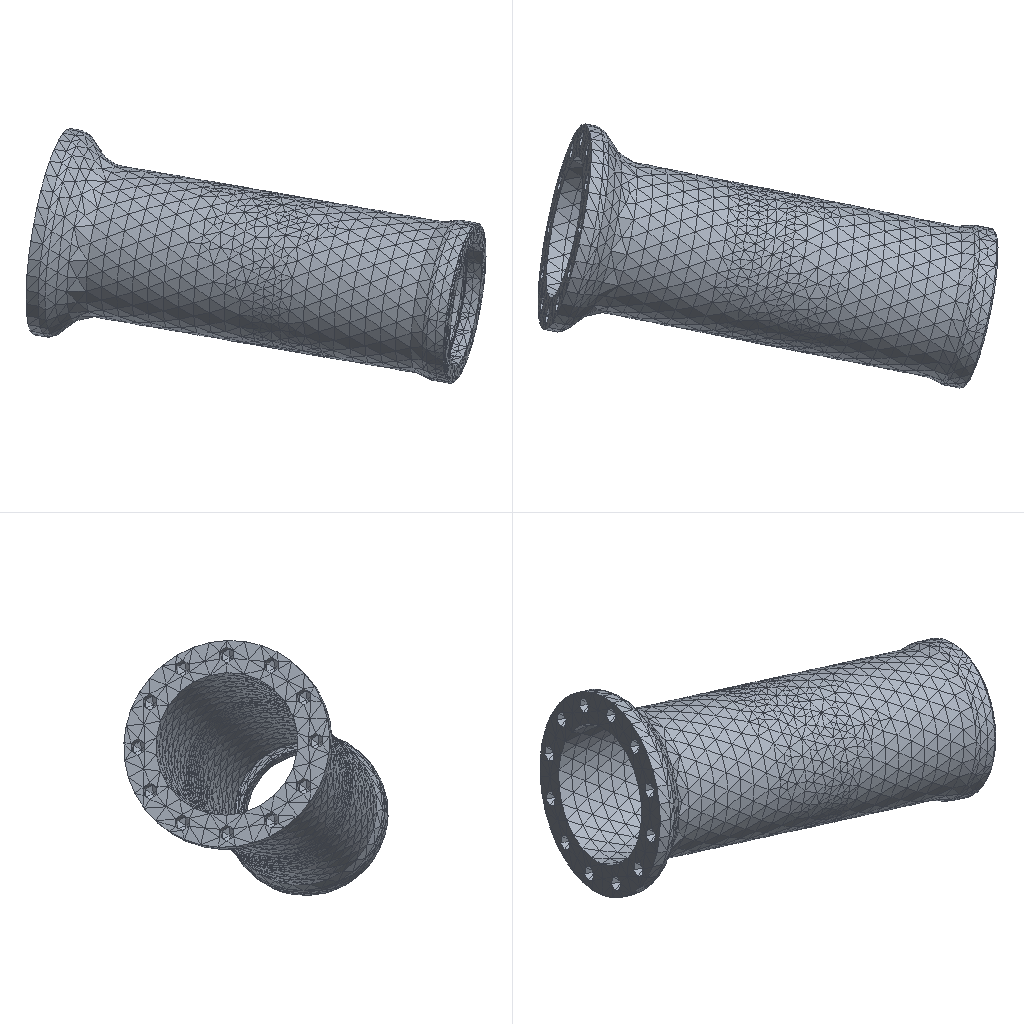Simulation study | ansys workbench
Set-up summary:
category,name,step,type,value,unit,region
solver,ansys_workbench
units,mm-N-s-tonne (MPa),,stated,"/units,MPA"
analysis,LS1,,transient
load_step,LS1,LS1,transient,time=0.171
mesh,nodes,,,3014
mesh,elements,,,9796
element_type,SOLID185,,,9455
element_type,CONTA174,,,341
material,moduan,,E,210000,tonne s^-2 mm^-1
material,moduan,,nu,0.3
material,moduan,,density,7.85e-09,tonne mm^-3
material,joint_1,,E,210000,tonne s^-2 mm^-1
material,joint_1,,nu,0.3
material,joint_1,,density,9.34279e-10,tonne mm^-3
material,link,,E,69000,tonne s^-2 mm^-1
material,link,,nu,0.3
material,link,,density,2.7e-09,tonne mm^-3
material,joint_4,,E,210000,tonne s^-2 mm^-1
material,joint_4,,nu,0.3
material,joint_4,,density,2.47283e-09,tonne mm^-3
material,joint_5,,E,210000,tonne s^-2 mm^-1
material,joint_5,,nu,0.3
material,joint_5,,density,1.91585e-09,tonne mm^-3
material,joint_6,,E,210000,tonne s^-2 mm^-1
material,joint_6,,nu,0.3
material,joint_6,,density,2.14316e-09,tonne mm^-3
material,joint_3,,E,210000,tonne s^-2 mm^-1
material,joint_3,,nu,0.3
material,joint_3,,density,1.46252e-09,tonne mm^-3
material,jpint_2,,E,210000,tonne s^-2 mm^-1
material,jpint_2,,nu,0.3
material,jpint_2,,density,1.01587e-08,tonne mm^-3
load,ACEL,LS1,gravity (ACEL; gravity acts opposite),"9806.65 [dir=(0, -1, 0)]",,all
bc,,LS1,fixed,"[dofs=ROTX,ROTY,ROTZ,UX,UY,UZ n=6]",,node list
contact,contact 1,,bonded (always),element=CONTA174
contact,contact 2,,bonded (always),element=CONTA174
named_set,REMOTEDISPALL,,node,1
Ansys APDL input file, long lists of numbers shortened:
/batch
/config,noeldb,1     ! force off writing results to database
*get,_wallstrt,active,,time,wall
! ANSYS input file written by Workbench version 2020 R2
! File used for geometry attach:
/title,UR16e--Transient (A5)
*DIM,_wb_ProjectScratch_dir,string,248
_wb_ProjectScratch_dir(1) = ''
*DIM,_wb_SolverFiles_dir,string,248
_wb_SolverFiles_dir(1) = ''
*DIM,_wb_userfiles_dir,string,248
_wb_userfiles_dir(1) = ''
/com,--- Data in consistent NMM units. See Solving Units in the help system for more information.
/units,MPA
/nopr
/wb,file,start              !  signify a WB generated input file
/prep7
! Turn off shape checking because checks already performed inside WB mesher.
! See help system for more information.
SHPP,OFF,,NOWARN
/nolist
etcon,set             ! allow ANSYS to choose best KEYOP's for 180x elements
/com,*********** Nodes for the whole assembly ***********
nblock,3,,3291
(1i9,3e20.9e3)
     2990    -2.619038221E+02     6.000698852E+02    -1.306205958E+02
! (2991 more lines like these left out)
-1
/com,*********** Nodes for all Remote Points ***********
nblock,3
(1i9,3e20.9e3)
   114271     1.429985942E-14     1.067999974E+02     1.194186063E-13
! (21 more lines like these left out)
-1
/wb,elem,start            !  set before creation of elements
/com,*********** Elements for Body 1 "base" ***********
/com,*********** Send Body as a Rigid Body ***********
et,1,21
keyo,1,2,1             ! Moments of inertia in nodal coordinates
keyo,1,3,0         ! 3D Mass With Rotary Intertia
r,1,1.02367975074938e-002,1.02367975074938e-002,1.02367975074938e-002,26.633,39.557,29.838
local,11,0,7.8090358886332e-002,63.831,-1.168,-0.1084,-3.09,0.1323
nrot,1
csys,0
mat,1
real,1
type,1
en,15078,1
/com,*********** Elements for Body 2 "joint_1" ***********
/com,*********** Send Body as a Rigid Body ***********
et,2,21
keyo,2,2,1             ! Moments of inertia in nodal coordinates
keyo,2,3,0         ! 3D Mass With Rotary Intertia
r,2,3.19999436398941e-003,3.19999436398941e-003,3.19999436398941e-003,13.065,11.645,10.957
local,11,0,-2.749,184.232,-15.857,-0.9454,5.268,9.901
nrot,2
csys,0
mat,2
real,2
type,2
en,15079,2
/com,*********** Elements for Body 3 "link_3" ***********
et,3,185
eblock,19,solid,,9455
(19i9)
        3        3        3        3        0        0        0        0        8        0        1      629     2969     1014     1014      630      630      630      630
! (9454 more lines like these left out)
-1
/com,*********** Elements for Body 4 "Link_2" ***********
/com,*********** Send Body as a Rigid Body ***********
et,4,21
keyo,4,2,1             ! Moments of inertia in nodal coordinates
keyo,4,3,0         ! 3D Mass With Rotary Intertia
r,4,8.50492430756376e-004,8.50492430756376e-004,8.50492430756376e-004,2.049,2.57,2.908
local,11,0,-233.317,606.482,-20.639,-10.872,-1.872,-37.264
nrot,2985
csys,0
mat,4
real,4
type,4
en,15080,2985
/com,*********** Elements for Body 5 "jpint_4" ***********
/com,*********** Send Body as a Rigid Body ***********
et,5,21
keyo,5,2,1             ! Moments of inertia in nodal coordinates
keyo,5,3,0         ! 3D Mass With Rotary Intertia
r,5,1.79999317481185e-003,1.79999317481185e-003,1.79999317481185e-003,2.575,2.69,2.136
local,11,0,99.549,541.334,-55.788,-10.802,-1.885,3.272
nrot,2986
csys,0
mat,5
real,5
type,5
en,15081,2986
/com,*********** Elements for Body 6 "joint_5" ***********
/com,*********** Send Body as a Rigid Body ***********
et,6,21
keyo,6,2,1             ! Moments of inertia in nodal coordinates
keyo,6,3,0         ! 3D Mass With Rotary Intertia
r,6,1.79999426944407e-003,1.79999426944407e-003,1.79999426944407e-003,3.487,3.061,2.341
local,11,0,83.755,539.911,-172.299,-41.598,-4.879,7.34
nrot,2987
csys,0
mat,6
real,6
type,6
en,15082,2987
/com,*********** Elements for Body 7 "joint_6" ***********
/com,*********** Send Body as a Rigid Body ***********
et,7,21
keyo,7,2,1             ! Moments of inertia in nodal coordinates
keyo,7,3,0         ! 3D Mass With Rotary Intertia
r,7,1.799990079675e-003,1.799990079675e-003,1.799990079675e-003,2.398,2.565,3.034
local,11,0,151.28,621.209,-202.996,36.251,5.214,7.789
nrot,2988
csys,0
mat,7
real,7
type,7
en,15083,2988
/com,*********** Elements for Body 8 "moduan" ***********
/com,*********** Send Body as a Rigid Body ***********
et,8,21
keyo,8,2,1             ! Moments of inertia in nodal coordinates
keyo,8,3,0         ! 3D Mass With Rotary Intertia
r,8,2.97368674504464e-003,2.97368674504464e-003,2.97368674504464e-003,2.801,2.33,2.336
local,11,0,220.284,574.903,-213.956,-38.665,-27.596,7.642
nrot,2989
csys,0
mat,8
real,8
type,8
en,15084,2989
/com,*********** Elements for Body 9 "joint_3" ***********
/com,*********** Send Body as a Rigid Body ***********
et,9,21
keyo,9,2,1             ! Moments of inertia in nodal coordinates
keyo,9,3,0         ! 3D Mass With Rotary Intertia
r,9,2.40005206162437e-003,2.40005206162437e-003,2.40005206162437e-003,5.964,5.358,4.799
local,11,0,-261.904,600.07,-130.621,32.525,-18.283,9.006
nrot,2990
csys,0
mat,9
real,9
type,9
en,15085,2990
/com,*********** Elements for Body 10 "joint_2" ***********
/com,*********** Send Body as a Rigid Body ***********
et,10,21
keyo,10,2,1             ! Moments of inertia in nodal coordinates
keyo,10,3,0         ! 3D Mass With Rotary Intertia
r,10,3.06619312289427e-002,3.06619312289427e-002,3.06619312289427e-002,112.393,110.597,96.78
local,11,0,-33.808,186.218,-176.77,27.519,12.66,8.86
nrot,2991
csys,0
mat,10
real,10
type,10
en,15086,2991
/com,*********** Elements for Body 11 "Link_1" ***********
/com,*********** Send Body as a Rigid Body ***********
et,11,21
keyo,11,2,1             ! Moments of inertia in nodal coordinates
keyo,11,3,0         ! 3D Mass With Rotary Intertia
r,11,2.24521379583667e-003,2.24521379583667e-003,2.24521379583667e-003,34.363,6.799,34.363
local,11,0,-138.935,377.254,-154.531,28.98,4.803,0.4433
nrot,2992
csys,0
mat,11
real,11
type,11
en,15087,2992
/wb,elem,end               !  done creating elements
/com,*********** Send User Defined Coordinate System(s) ***********
local,12,0,1.42998594161399e-014,106.8,1.19418606342056e-013,5.518,-90.,5.518
local,13,0,-17.447,180.7,-100.598,-1.26833640216353e-014,9.7869357942221e-014,9.839
local,14,0,-255.778,609.325,-64.845,-1.19904740548723e-015,4.20102064352059e-013,9.839
local,15,0,95.681,540.401,-106.111,-7.6091083357917e-015,1.34257806861156e-013,9.839
local,16,0,113.452,577.213,-196.426,180.,-81.305,-138.924
local,17,0,196.105,596.769,-210.196,-180.,80.114,-132.6
local,18,0,-68.796,250.612,-166.696,99.269,-76.01,69.735
local,19,0,-231.933,545.166,-138.402,-1.12265577235347e-013,-84.513,-28.868
local,20,0,-175.359,595.732,-8.966,173.246,24.487,-100.62
local,21,0,52.965,550.529,-48.565,-180.,48.78,-104.746
local,22,0,240.749,556.326,-217.244,-87.35,80.633,135.561
csys,0
toffst,273.15,  ! Temperature offset from absolute zero
/com,*********** Set Reference Temperature ***********
tref,22.
/wb,mat,start              !  starting to send materials
/com,*********** Send Materials ***********
MP,DENS,1,7.85e-09,	! tonne mm^-3
MP,EX,1,210000,	! tonne s^-2 mm^-1
MP,NUXY,1,0.3,
MP,DENS,2,9.34279e-10,	! tonne mm^-3
! (29 more lines like these left out)
/wb,mat,end                !  done sending materials
!************************* Model Summary ********************
!base,	moduan,	matid,	1
!joint_1,	joint_1,	matid,	2
!link_3,	link,	matid,	3
!Link_2,	link,	matid,	4
!jpint_4,	joint_4,	matid,	5
!joint_5,	joint_5,	matid,	6
!joint_6,	joint_6,	matid,	7
!moduan,	moduan,	matid,	8
!joint_3,	joint_3,	matid,	9
!joint_2,	jpint_2,	matid,	10
!Link_1,	link,	matid,	11
!************************* End Model Summary ********************
! get the diagonal of the bounding box. Needed later for other things
*get,_xmin,node,,mnloc,x
*get,_ymin,node,,mnloc,y
*get,_zmin,node,,mnloc,z
*get,_xmax,node,,mxloc,x
*get,_ymax,node,,mxloc,y
*get,_zmax,node,,mxloc,z
_ASMDIAG=(_xmax-_xmin)*(_xmax-_xmin)+(_ymax-_ymin)*(_ymax-_ymin)+(_zmax-_zmin)*(_zmax-_zmin)
_ASMDIAG=SQRT(_ASMDIAG)
/wb,contact,start          !  starting to send contact
/wb,contact,end            !  done creating contacts
/golist
/wb,load,start             !  starting to send loads
/com,*********** Create Remote Point "Internal Remote Point" ***********
! -------- Remote Point Used by "Revolute - base To joint_1" --------
! ********* Create Contact to Connect To Rigid Body Mass Node ***********
*set,tid,12
*set,cid,12
et,tid,170
keyo,tid,2,1           ! Set MPC target element and not fix pilot
keyo,tid,4,0           ! Create CE's for all DOFs
type,tid
mat ,cid
real,cid
tshape,pilo
en,613392,1
tshape
! ********* End of Create Contact to Connect To Rigid Body Mass Node ***********
*set,_npilot,114271
_npilot109=_npilot
mat,12
real,12
type,12
en,613393,1,114271
csys,12
nrot,114271
csys,0
/com,*********** Create Remote Point "Internal Remote Point 2" ***********
! -------- Remote Point Used by "Revolute - base To joint_1" --------
! ********* Create Contact to Connect To Rigid Body Mass Node ***********
*set,tid,13
*set,cid,13
et,tid,170
keyo,tid,2,1           ! Set MPC target element and not fix pilot
keyo,tid,4,0           ! Create CE's for all DOFs
type,tid
mat ,cid
real,cid
tshape,pilo
en,613394,2
tshape
! ********* End of Create Contact to Connect To Rigid Body Mass Node ***********
*set,_npilot,114272
_npilot110=_npilot
mat,13
real,13
type,13
en,613395,2,114272
csys,12
nrot,114272
csys,0
/com,*********** Create Remote Point "Internal Remote Point 3" ***********
! -------- Remote Point Used by "Revolute - joint_1 To joint_2" --------
*set,_npilot,114273
_npilot113=_npilot
mat,13
real,13
type,13
en,613396,2,114273
csys,13
nrot,114273
csys,0
/com,*********** Create Remote Point "Internal Remote Point 4" ***********
! -------- Remote Point Used by "Revolute - joint_1 To joint_2" --------
! ********* Create Contact to Connect To Rigid Body Mass Node ***********
*set,tid,14
*set,cid,14
et,tid,170
keyo,tid,2,1           ! Set MPC target element and not fix pilot
keyo,tid,4,0           ! Create CE's for all DOFs
type,tid
mat ,cid
real,cid
tshape,pilo
en,613397,2991
tshape
! ********* End of Create Contact to Connect To Rigid Body Mass Node ***********
*set,_npilot,114274
_npilot114=_npilot
mat,14
real,14
type,14
en,613398,2991,114274
csys,13
nrot,114274
csys,0
/com,*********** Create Remote Point "Internal Remote Point 5" ***********
! -------- Remote Point Used by "Revolute - joint_3 To Link_2" --------
! ********* Create Contact to Connect To Rigid Body Mass Node ***********
*set,tid,15
*set,cid,15
et,tid,170
keyo,tid,2,1           ! Set MPC target element and not fix pilot
keyo,tid,4,0           ! Create CE's for all DOFs
type,tid
mat ,cid
real,cid
tshape,pilo
en,613399,2990
tshape
! ********* End of Create Contact to Connect To Rigid Body Mass Node ***********
*set,_npilot,114275
_npilot117=_npilot
mat,15
real,15
type,15
en,613400,2990,114275
csys,14
nrot,114275
csys,0
/com,*********** Create Remote Point "Internal Remote Point 6" ***********
! -------- Remote Point Used by "Revolute - joint_3 To Link_2" --------
! ********* Create Contact to Connect To Rigid Body Mass Node ***********
*set,tid,16
*set,cid,16
et,tid,170
keyo,tid,2,1           ! Set MPC target element and not fix pilot
keyo,tid,4,0           ! Create CE's for all DOFs
type,tid
mat ,cid
real,cid
tshape,pilo
en,613401,2985
tshape
! ********* End of Create Contact to Connect To Rigid Body Mass Node ***********
*set,_npilot,114276
_npilot118=_npilot
mat,16
real,16
type,16
en,613402,2985,114276
csys,14
nrot,114276
csys,0
/com,*********** Create Remote Point "Internal Remote Point 7" ***********
! -------- Remote Point Used by "Revolute - jpint_4 To joint_5" --------
! ********* Create Contact to Connect To Rigid Body Mass Node ***********
*set,tid,17
*set,cid,17
et,tid,170
keyo,tid,2,1           ! Set MPC target element and not fix pilot
keyo,tid,4,0           ! Create CE's for all DOFs
type,tid
mat ,cid
real,cid
tshape,pilo
en,613403,2986
tshape
! ********* End of Create Contact to Connect To Rigid Body Mass Node ***********
*set,_npilot,114277
_npilot121=_npilot
mat,17
real,17
type,17
en,613404,2986,114277
csys,15
nrot,114277
csys,0
/com,*********** Create Remote Point "Internal Remote Point 8" ***********
! -------- Remote Point Used by "Revolute - jpint_4 To joint_5" --------
! ********* Create Contact to Connect To Rigid Body Mass Node ***********
*set,tid,18
*set,cid,18
et,tid,170
keyo,tid,2,1           ! Set MPC target element and not fix pilot
keyo,tid,4,0           ! Create CE's for all DOFs
type,tid
mat ,cid
real,cid
tshape,pilo
en,613405,2987
tshape
! ********* End of Create Contact to Connect To Rigid Body Mass Node ***********
*set,_npilot,114278
_npilot122=_npilot
mat,18
real,18
type,18
en,613406,2987,114278
csys,15
nrot,114278
csys,0
/com,*********** Create Remote Point "Internal Remote Point 9" ***********
! -------- Remote Point Used by "Revolute - joint_5 To joint_6" --------
*set,_npilot,114279
_npilot125=_npilot
mat,18
real,18
type,18
en,613407,2987,114279
csys,16
nrot,114279
csys,0
/com,*********** Create Remote Point "Internal Remote Point 10" ***********
! -------- Remote Point Used by "Revolute - joint_5 To joint_6" --------
! ********* Create Contact to Connect To Rigid Body Mass Node ***********
*set,tid,19
*set,cid,19
et,tid,170
keyo,tid,2,1           ! Set MPC target element and not fix pilot
keyo,tid,4,0           ! Create CE's for all DOFs
type,tid
mat ,cid
real,cid
tshape,pilo
en,613408,2988
tshape
! ********* End of Create Contact to Connect To Rigid Body Mass Node ***********
*set,_npilot,114280
_npilot126=_npilot
mat,19
real,19
type,19
en,613409,2988,114280
csys,16
nrot,114280
csys,0
/com,*********** Create Remote Point "Internal Remote Point 11" ***********
! -------- Remote Point Used by "Revolute - joint_6 To moduan" --------
*set,_npilot,114281
_npilot129=_npilot
mat,19
real,19
type,19
en,613410,2988,114281
csys,17
nrot,114281
csys,0
/com,*********** Create Remote Point "Internal Remote Point 12" ***********
! -------- Remote Point Used by "Revolute - joint_6 To moduan" --------
! ********* Create Contact to Connect To Rigid Body Mass Node ***********
*set,tid,20
*set,cid,20
et,tid,170
keyo,tid,2,1           ! Set MPC target element and not fix pilot
keyo,tid,4,0           ! Create CE's for all DOFs
type,tid
mat ,cid
real,cid
tshape,pilo
en,613411,2989
tshape
! ********* End of Create Contact to Connect To Rigid Body Mass Node ***********
*set,_npilot,114282
_npilot130=_npilot
mat,20
real,20
type,20
en,613412,2989,114282
csys,17
nrot,114282
csys,0
/com,*********** Create Remote Point "Internal Remote Point 13" ***********
! -------- Remote Point Used by "Fixed - joint_2 To Link_1" --------
*set,_npilot,114283
_npilot158=_npilot
mat,14
real,14
type,14
en,613413,2991,114283
csys,18
nrot,114283
csys,0
/com,*********** Create Remote Point "Internal Remote Point 14" ***********
! -------- Remote Point Used by "Fixed - joint_2 To Link_1" --------
! ********* Create Contact to Connect To Rigid Body Mass Node ***********
*set,tid,21
*set,cid,21
et,tid,170
keyo,tid,2,1           ! Set MPC target element and not fix pilot
keyo,tid,4,0           ! Create CE's for all DOFs
type,tid
mat ,cid
real,cid
tshape,pilo
en,613414,2992
tshape
! ********* End of Create Contact to Connect To Rigid Body Mass Node ***********
*set,_npilot,114284
_npilot159=_npilot
mat,21
real,21
type,21
en,613415,2992,114284
csys,18
nrot,114284
csys,0
/com,*********** Create Remote Point "Internal Remote Point 15" ***********
! -------- Remote Point Used by "Fixed - Link_1 To joint_3" --------
*set,_npilot,114285
_npilot162=_npilot
mat,21
real,21
type,21
en,613416,2992,114285
csys,19
nrot,114285
csys,0
/com,*********** Create Remote Point "Internal Remote Point 16" ***********
! -------- Remote Point Used by "Fixed - Link_1 To joint_3" --------
*set,_npilot,114286
_npilot163=_npilot
mat,15
real,15
type,15
en,613417,2990,114286
csys,19
nrot,114286
csys,0
/com,*********** Create Remote Point "Internal Remote Point 17" ***********
! -------- Remote Point Used by "Fixed - Link_2 To link_3" --------
*set,_npilot,114287
_npilot166=_npilot
mat,16
real,16
type,16
en,613418,2985,114287
csys,20
nrot,114287
csys,0
/com,*********** Create Remote Point "Internal Remote Point 18" ***********
! -------- Remote Point Used by "Fixed - Link_2 To link_3" --------
*set,tid,23
*set,cid,22
et,cid,174
et,tid,170
keyo,tid,2,1               ! Don't fix the pilot node
keyo,tid,4,0               ! Activate all DOF's due to large deformation
keyo,cid,12,5              ! Bonded Contact
keyo,cid,4,2               ! Rigid CERIG style load
keyo,cid,2,2               ! MPC style contact
eblock,10,,,183
(15i9)
   613419       22       22       22        0      168      173      191      191
! (182 more lines like these left out)
-1
*set,_npilot,114288
_npilot167=_npilot
type,tid
mat ,cid
real,cid
tshape,pilo
en,613602,_npilot
tshape
csys,20
nrot,114288
csys,0
/com,*********** Create Remote Point "Internal Remote Point 19" ***********
! -------- Remote Point Used by "Fixed - link_3 To jpint_4" --------
*set,tid,25
*set,cid,24
et,cid,174
et,tid,170
keyo,tid,2,1               ! Don't fix the pilot node
keyo,tid,4,0               ! Activate all DOF's due to large deformation
keyo,cid,12,5              ! Bonded Contact
keyo,cid,4,2               ! Rigid CERIG style load
keyo,cid,2,2               ! MPC style contact
eblock,10,,,158
(15i9)
   613603       24       24       24        0      636      541      637      637
! (157 more lines like these left out)
-1
*set,_npilot,114289
_npilot170=_npilot
type,tid
mat ,cid
real,cid
tshape,pilo
en,613761,_npilot
tshape
csys,21
nrot,114289
csys,0
/com,*********** Create Remote Point "Internal Remote Point 20" ***********
! -------- Remote Point Used by "Fixed - link_3 To jpint_4" --------
*set,_npilot,114290
_npilot171=_npilot
mat,17
real,17
type,17
en,613762,2986,114290
csys,21
nrot,114290
csys,0
/com,*********** Create Remote Point "Internal Remote Point 21" ***********
! -------- Remote Point Used by "Remote Displacement" --------
*set,_npilot,114291
_npilot196=_npilot
mat,12
real,12
type,12
en,613763,1,114291
/com,*********** Create Remote Point "Internal Remote Point 22" ***********
! -------- Remote Point Used by "Point Mass" --------
*set,_npilot,114292
_npilot211=_npilot
mat,20
real,20
type,20
en,613764,2989,114292
csys,22
nrot,114292
csys,0
/com,*********** Construct Remote Displacement ***********
/COM,*** Create a component for all remote displacements ***
CMBLOCK,REMOTEDISPALL,NODE,        1
(8i10)
    114291
/com,*********** Construct Remote Mass Using Remote Attachment ***********
*set,_tid,26
et,_tid,21           ! MASS21 element
type,_tid
mat ,_tid
real,_tid
keyo,_tid,3,2        ! 3d mass without rotary inertia
r,_tid,1.6e-002
en,613765,114292
/com,*********** Create Joint "Revolute - base To joint_1" ***********
/com,            Real Constant Set For Above Joint Is 27
! Joint Element Type Declaration and Definition using MPC184
*set,_jid,27
et,_jid,184
keyo,_jid,1,6           ! Revolute Joint
keyo,_jid,4,1           ! Z Axis is revolute axis
sectype,_jid, joint, revo, _wbjoint
secjoint,,12,12
mat,_jid
real,_jid
type,_jid
secnum,_jid
en,613360,114271,114272      ! body to body joint
/com,*********** Create Joint "Revolute - joint_1 To joint_2" ***********
/com,            Real Constant Set For Above Joint Is 28
! Joint Element Type Declaration and Definition using MPC184
*set,_jid,28
et,_jid,184
keyo,_jid,1,6           ! Revolute Joint
keyo,_jid,4,1           ! Z Axis is revolute axis
sectype,_jid, joint, revo, _wbjoint
secjoint,,13,13
mat,_jid
real,_jid
type,_jid
secnum,_jid
en,613361,114273,114274      ! body to body joint
/com,*********** Create Joint "Revolute - joint_3 To Link_2" ***********
/com,            Real Constant Set For Above Joint Is 29
! Joint Element Type Declaration and Definition using MPC184
*set,_jid,29
et,_jid,184
keyo,_jid,1,6           ! Revolute Joint
keyo,_jid,4,1           ! Z Axis is revolute axis
sectype,_jid, joint, revo, _wbjoint
secjoint,,14,14
mat,_jid
real,_jid
type,_jid
secnum,_jid
en,613362,114275,114276      ! body to body joint
/com,*********** Create Joint "Revolute - jpint_4 To joint_5" ***********
/com,            Real Constant Set For Above Joint Is 30
! Joint Element Type Declaration and Definition using MPC184
*set,_jid,30
et,_jid,184
keyo,_jid,1,6           ! Revolute Joint
keyo,_jid,4,1           ! Z Axis is revolute axis
sectype,_jid, joint, revo, _wbjoint
secjoint,,15,15
mat,_jid
real,_jid
type,_jid
secnum,_jid
en,613363,114277,114278      ! body to body joint
/com,*********** Create Joint "Revolute - joint_5 To joint_6" ***********
/com,            Real Constant Set For Above Joint Is 31
! Joint Element Type Declaration and Definition using MPC184
*set,_jid,31
et,_jid,184
keyo,_jid,1,6           ! Revolute Joint
keyo,_jid,4,1           ! Z Axis is revolute axis
sectype,_jid, joint, revo, _wbjoint
secjoint,,16,16
mat,_jid
real,_jid
type,_jid
secnum,_jid
en,613364,114279,114280      ! body to body joint
/com,*********** Create Joint "Revolute - joint_6 To moduan" ***********
/com,            Real Constant Set For Above Joint Is 32
! Joint Element Type Declaration and Definition using MPC184
*set,_jid,32
et,_jid,184
keyo,_jid,1,6           ! Revolute Joint
keyo,_jid,4,1           ! Z Axis is revolute axis
sectype,_jid, joint, revo, _wbjoint
secjoint,,17,17
mat,_jid
real,_jid
type,_jid
secnum,_jid
en,613365,114281,114282      ! body to body joint
/com,*********** Create Joint "Fixed - joint_2 To Link_1" ***********
! Joint Element Type Declaration and Definition using CONTACT
*set,tid,33
*set,cid,33
et,tid,170
keyo,tid,2,1           ! Set MPC target element and not fix pilot
keyo,tid,4,0           ! Create CE's for all DOFs
mat,cid
real,cid
type,tid
tshape,pilo
en,613366,114283        ! create pilot node for rigid link
tshape
type,cid
en,613766,114283,114284      ! body to body joint
csys,0
/com,*********** Create Joint "Fixed - Link_1 To joint_3" ***********
! Joint Element Type Declaration and Definition using CONTACT
*set,tid,34
*set,cid,34
et,tid,170
keyo,tid,2,1           ! Set MPC target element and not fix pilot
keyo,tid,4,0           ! Create CE's for all DOFs
mat,cid
real,cid
type,tid
tshape,pilo
en,613367,114285        ! create pilot node for rigid link
tshape
type,cid
en,613767,114285,114286      ! body to body joint
csys,0
/com,*********** Create Joint "Fixed - Link_2 To link_3" ***********
! Joint Element Type Declaration and Definition using CONTACT
*set,tid,35
*set,cid,35
et,tid,170
keyo,tid,2,1           ! Set MPC target element and not fix pilot
keyo,tid,4,0           ! Create CE's for all DOFs
mat,cid
real,cid
type,tid
tshape,pilo
en,613368,114287        ! create pilot node for rigid link
tshape
type,cid
en,613768,114287,114288      ! body to body joint
csys,0
/com,*********** Create Joint "Fixed - link_3 To jpint_4" ***********
! Joint Element Type Declaration and Definition using CONTACT
*set,tid,36
*set,cid,36
et,tid,170
keyo,tid,2,1           ! Set MPC target element and not fix pilot
keyo,tid,4,0           ! Create CE's for all DOFs
mat,cid
real,cid
type,tid
tshape,pilo
en,613369,114289        ! create pilot node for rigid link
tshape
type,cid
en,613769,114289,114290      ! body to body joint
csys,0
/com,*********** Create Joint Drivers **********
*DIM,_loadvari200,TABLE,301,1,1,TIME,
! Time values
_loadvari200(1,0,1) = 0.
_loadvari200(2,0,1) = 9.e-003
! (299 more lines like these left out)
! Load values
_loadvari200(1,1,1) = 0.
_loadvari200(2,1,1) = 1.11781880872004e-002
! (299 more lines like these left out)
*DIM,_loadvari201,TABLE,301,1,1,TIME,
! Time values
_loadvari201(1,0,1) = 0.
_loadvari201(2,0,1) = 9.e-003
! (299 more lines like these left out)
! Load values
_loadvari201(1,1,1) = 0.
_loadvari201(2,1,1) = 9.42474305418434e-003
! (299 more lines like these left out)
*DIM,_loadvari202,TABLE,301,1,1,TIME,
! Time values
_loadvari202(1,0,1) = 0.
_loadvari202(2,0,1) = 9.e-003
! (299 more lines like these left out)
! Load values
_loadvari202(1,1,1) = 0.
_loadvari202(2,1,1) = 6.20279544183273e-003
! (299 more lines like these left out)
*DIM,_loadvari203,TABLE,301,1,1,TIME,
! Time values
_loadvari203(1,0,1) = 0.
_loadvari203(2,0,1) = 9.e-003
! (299 more lines like these left out)
! Load values
_loadvari203(1,1,1) = 0.
_loadvari203(2,1,1) = 5.74251721149678e-003
! (299 more lines like these left out)
*DIM,_loadvari204,TABLE,301,1,1,TIME,
! Time values
_loadvari204(1,0,1) = 0.
_loadvari204(2,0,1) = 9.e-003
! (299 more lines like these left out)
! Load values
_loadvari204(1,1,1) = 0.
_loadvari204(2,1,1) = 6.80554489900897e-003
! (299 more lines like these left out)
*DIM,_loadvari205,TABLE,301,1,1,TIME,
! Time values
_loadvari205(1,0,1) = 0.
_loadvari205(2,0,1) = 9.e-003
! (299 more lines like these left out)
! Load values
_loadvari205(1,1,1) = 0.
_loadvari205(2,1,1) = 8.88775760322324e-003
! (299 more lines like these left out)
/gst,on,on
fini
*get,_numnode,node,0,count
*get,_numelem,elem,0,count
*get, _MAXELEMNUM, elem, 0, NUM, MAX
*get, _MAXNODENUM, node, 0, NUM, MAX
*get, _MAXELEMTYPE, etyp, 0, NUM, MAX
*get, _MAXREALCONST, real, 0, NUM, MAX
/go
/wb,load,end               !  done creating loads
/com,--- Number of total nodes = %_numnode%
/com,--- Number of contact elements = 341
/com,--- Number of spring elements = 0
/com,--- Number of bearing elements = 0
/com,--- Number of solid elements = 9465
/com,--- Number of condensed parts = 0
/com,--- Number of total elements = %_numelem%
*get,_wallbsol,active,,time,wall
/com,****************************************************************************
/com,*************************    SOLUTION       ********************************
/com,****************************************************************************
/solu
antype,4                   ! transient analysis
nlgeom,on                  ! Turn on Large Deformation Effects
kbc,1                      ! stepped BC's
_thickRatio=  0     ! Ratio of thick parts in the model
eqsl,sparse,,,,,1
cntr,print,1               ! print out contact info and also make no initial contact an error
dmpoption,emat,no             ! Don't combine emat file for DANSYS
dmpoption,esav,no             ! Don't combine esav file for DANSYS
trnopt,full,,,,,hht        ! HHT time integration method
tintp, mosp			! Choose transient integration settings for moderate speed application
nldiag,cont,iter           ! print out contact info each equilibrium iteration
rescontrol,define,last,last,,dele	   ! Program Controlled
/com,****************************************************
/com,******************* SOLVE FOR LS 1 OF 1 ****************
d,114291,ux,0.
d,114291,uy,0.
d,114291,uz,0.
d,114291,rotx,0.
d,114291,roty,0.
d,114291,rotz,0.
acel,0.,9806.65,0.
/nopr
/gopr
esel,s,type,,27
dj,all,rotz,%_loadvari200%
esel,all
esel,s,type,,28
dj,all,rotz,%_loadvari201%
esel,all
esel,s,type,,29
dj,all,rotz,%_loadvari202%
esel,all
esel,s,type,,30
dj,all,rotz,%_loadvari203%
esel,all
esel,s,type,,31
dj,all,rotz,%_loadvari204%
esel,all
esel,s,type,,32
dj,all,rotz,%_loadvari205%
esel,all
autots,on                   ! User turned on automatic time stepping
deltim,0.009,0.009,0.009,OFF
time,0.171
timint,on                  ! Turn on time integration effects
outres,erase
outres,all,none
outres,nsol,all,
outres,rsol,all
outres,eangl,all
outres,etmp,all
outres,veng,all
outres,strs,all,
outres,epel,all,
outres,eppl,all,
outres,cont,all,
outres,v,all,
outres,a,all,
/nopr
esel,s,type,,1
esel,a,type,,2
esel,a,type,,4,11
esel,a,type,,27,32
cm,_elmisc,elem
esel,all
/gopr
outres,misc,all,_elmisc
! *********** WB SOLVE COMMAND ***********
! check interactive state
*get,ANSINTER_,active,,int
*if,ANSINTER_,ne,0,then
/eof
*endif
solve
/com *************** Write FE CONNECTORS *********
CEWRITE,file,ce,,INTE
/com,****************************************************
/com,*************** FINISHED SOLVE FOR LS 1 *************
*get,_wallasol,active,,time,wall
/nopr
*get,_numnode,node,0,count
*get,_numelem,elem,0,count
*get, _MAXELEMNUM, elem, 0, NUM, MAX
*get, _MAXNODENUM, node, 0, NUM, MAX,,,INTERNAL
*get, _MAXELEMTYPE, etyp, 0, NUM, MAX
*get, _MAXREALCONST, real, 0, NUM, MAX
/gopr
/post1
xmlo,ENCODING,ISO-8859-1
xmlo,parm
/xml,parm,xml
fini
/gopr
*get,_walldone,active,,time,wall
_preptime=(_wallbsol-_wallstrt)*3600
_solvtime=(_wallasol-_wallbsol)*3600
_posttime=(_walldone-_wallasol)*3600
_totaltim=(_walldone-_wallstrt)*3600
*get,_dlbratio,active,0,solu,dlbr
*get,_combtime,active,0,solu,comb
/com,--- Total number of nodes = %_numnode%
/com,--- Total number of elements = %_numelem%
/com,--- Element load balance ratio = %_dlbratio%
/com,--- Time to combine distributed files = %_combtime%
/wb,file,end               ! done with WB generated input
Results summary:
result,analyses[0].index,,,1
result,analyses[0].system,,,SYS
result,analyses[0].deck,,,deck.dat
result,analyses[0].solve_status,,,completed
result,analyses[0].analysis_type,,,static
result,analyses[0].physics,,,mechanical
result,analyses[0].unit_system,,,"NMM: mm, ton, N, s, mV, mA, degC"
result,analyses[0].n_sets,,,19
result,analyses[0].load_steps[0].set,set=19,,19
result,analyses[0].load_steps[0].time_or_freq,set=19,,0.171
result,analyses[0].load_steps[0].max_displacement_magnitude,set=19,,2220.55
result,analyses[0].load_steps[0].max_von_mises_nodal,set=19,,71.822
result,analyses[0].load_steps[0].reaction_force_sum_xyz[1],set=19,,-1058.54
result,analyses[0].load_steps[0].reaction_force_sum_xyz[2],set=19,,-1292.74
result,analyses[0].load_steps[0].reaction_force_sum_xyz[3],set=19,,1348.65
result,geometry_export[0][0],,,.step
result,geometry_export[0][1],,,ok
result,geometry_export[0][2],,,11